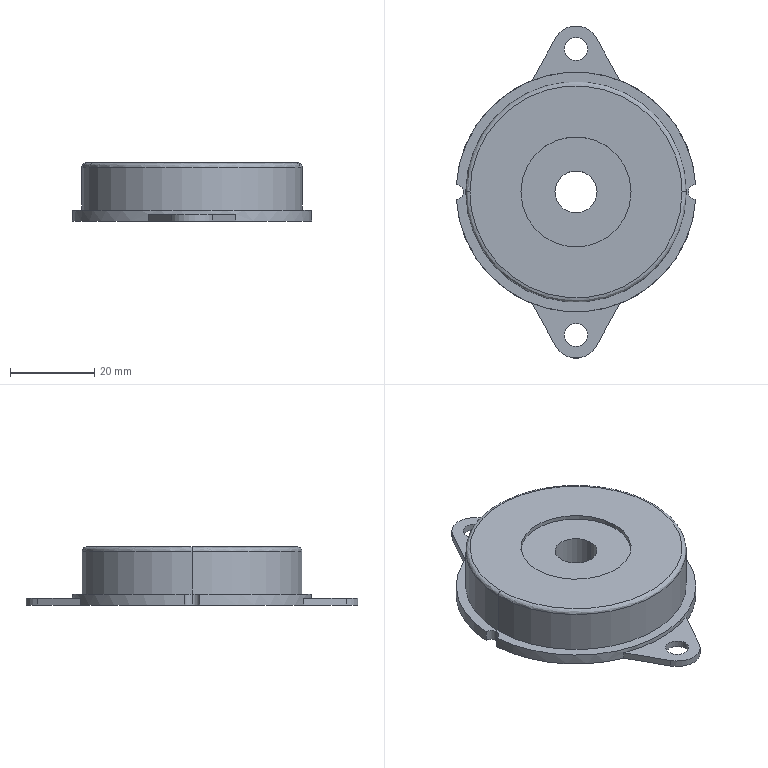Part | SolidWorks | features BaseBody 1 | 1 solid | 32 faces | box 56.886 x 79 x 13.8 mm | volume 28746 mm3 | cylinder 19 | plane 11 | spline 2 | commonest cylinder face diameters 5.5 x4 26.2 x4 3.6 x3 10 x2 11 x2 52.4 x2
STEP:
#1=CARTESIAN_POINT('',(26.2,0.,12.8));
#2=VERTEX_POINT('',#1);
#3=CARTESIAN_POINT('',(-26.2,0.,12.8));
#4=VERTEX_POINT('',#3);
#5=CARTESIAN_POINT('',(0.,0.,12.8));
#6=DIRECTION('',(0.,0.,-1.));
#7=DIRECTION('',(-1.,0.,0.));
#8=AXIS2_PLACEMENT_3D('',#5,#6,#7);
#9=CIRCLE('',#8,26.2);
#10=EDGE_CURVE('',#2,#4,#9,.T.);
#11=ORIENTED_EDGE('',*,*,#10,.F.);
#12=CARTESIAN_POINT('',(25.2,0.,13.8));
#13=VERTEX_POINT('',#12);
#14=CARTESIAN_POINT('',(25.2,0.,12.8));
#15=DIRECTION('',(0.,-1.,0.));
#16=DIRECTION('',(1.,0.,0.));
#17=AXIS2_PLACEMENT_3D('',#14,#15,#16);
#18=CIRCLE('',#17,1.);
#19=EDGE_CURVE('',#2,#13,#18,.T.);
#20=ORIENTED_EDGE('',*,*,#19,.T.);
#21=CARTESIAN_POINT('',(-25.2,0.,13.8));
#22=VERTEX_POINT('',#21);
#23=CARTESIAN_POINT('',(25.2,0.,13.8));
#24=CARTESIAN_POINT('',(25.2,-50.4,13.8));
#25=CARTESIAN_POINT('',(-25.2,-50.4,13.8));
#26=CARTESIAN_POINT('',(-25.2,0.,13.8));
#27=(BOUNDED_CURVE()B_SPLINE_CURVE(3,(#23,#24,#25,#26),.UNSPECIFIED.,.F.,.F.)B_SPLINE_CURVE_WITH_KNOTS((4,4),(0.5,1.),.UNSPECIFIED.)CURVE()GEOMETRIC_REPRESENTATION_ITEM()RATIONAL_B_SPLINE_CURVE((1.,0.3333,0.3333,1.))REPRESENTATION_ITEM(''));
#28=EDGE_CURVE('',#13,#22,#27,.T.);
#29=ORIENTED_EDGE('',*,*,#28,.T.);
#30=CARTESIAN_POINT('',(-25.2,0.,12.8));
#31=DIRECTION('',(0.,1.,0.));
#32=DIRECTION('',(-1.,0.,0.));
#33=AXIS2_PLACEMENT_3D('',#30,#31,#32);
#34=CIRCLE('',#33,1.);
#35=EDGE_CURVE('',#4,#22,#34,.T.);
#36=ORIENTED_EDGE('',*,*,#35,.F.);
#37=EDGE_LOOP('',(#11,#20,#29,#36));
#38=FACE_OUTER_BOUND('',#37,.T.);
#39=CARTESIAN_POINT('',(26.2,0.,12.8));
#40=CARTESIAN_POINT('',(26.2,-52.4,12.8));
#41=CARTESIAN_POINT('',(-26.2,-52.4,12.8));
#42=CARTESIAN_POINT('',(-26.2,0.,12.8));
#43=CARTESIAN_POINT('',(26.2,0.,13.386));
#44=CARTESIAN_POINT('',(26.2,-52.4,13.386));
#45=CARTESIAN_POINT('',(-26.2,-52.4,13.386));
#46=CARTESIAN_POINT('',(-26.2,0.,13.386));
#47=CARTESIAN_POINT('',(25.786,0.,13.8));
#48=CARTESIAN_POINT('',(25.786,-51.572,13.8));
#49=CARTESIAN_POINT('',(-25.786,-51.572,13.8));
#50=CARTESIAN_POINT('',(-25.786,0.,13.8));
#51=CARTESIAN_POINT('',(25.2,0.,13.8));
#52=CARTESIAN_POINT('',(25.2,-50.4,13.8));
#53=CARTESIAN_POINT('',(-25.2,-50.4,13.8));
#54=CARTESIAN_POINT('',(-25.2,0.,13.8));
#55=(BOUNDED_SURFACE()B_SPLINE_SURFACE(3,3,((#39,#40,#41,#42),(#43,#44,#45,#46),(#47,#48,#49,#50),(#51,#52,#53,#54)),.UNSPECIFIED.,.F.,.F.,.T.)B_SPLINE_SURFACE_WITH_KNOTS((4,4),(4,4),(0.,1.),(0.,1.),.UNSPECIFIED.)GEOMETRIC_REPRESENTATION_ITEM()RATIONAL_B_SPLINE_SURFACE(((1.,0.3333,0.3333,1.),(0.8047,0.2682,0.2682,0.8047),(0.8047,0.2682,0.2682,0.8047),(1.,0.3333,0.3333,1.)))REPRESENTATION_ITEM('')SURFACE());
#56=ADVANCED_FACE('',(#38),#55,.T.);
#57=CARTESIAN_POINT('',(-26.7,0.,0.));
#58=VERTEX_POINT('',#57);
#59=CARTESIAN_POINT('',(-28.443,1.799,0.));
#60=VERTEX_POINT('',#59);
#61=CARTESIAN_POINT('',(-28.5,0.,0.));
#62=DIRECTION('',(0.,0.,1.));
#63=DIRECTION('',(1.,0.,0.));
#64=AXIS2_PLACEMENT_3D('',#61,#62,#63);
#65=CIRCLE('',#64,1.8);
#66=EDGE_CURVE('',#58,#60,#65,.T.);
#67=ORIENTED_EDGE('',*,*,#66,.F.);
#68=CARTESIAN_POINT('',(-26.7,0.,2.6));
#69=VERTEX_POINT('',#68);
#70=CARTESIAN_POINT('',(-26.7,0.,-86.643));
#71=DIRECTION('',(0.,0.,1.));
#72=VECTOR('',#71,1000.);
#73=LINE('',#70,#72);
#74=EDGE_CURVE('',#58,#69,#73,.T.);
#75=ORIENTED_EDGE('',*,*,#74,.T.);
#76=CARTESIAN_POINT('',(-28.443,1.799,2.6));
#77=VERTEX_POINT('',#76);
#78=CARTESIAN_POINT('',(-28.5,0.,2.6));
#79=DIRECTION('',(0.,0.,-1.));
#80=DIRECTION('',(1.,0.,0.));
#81=AXIS2_PLACEMENT_3D('',#78,#79,#80);
#82=CIRCLE('',#81,1.8);
#83=EDGE_CURVE('',#77,#69,#82,.T.);
#84=ORIENTED_EDGE('',*,*,#83,.F.);
#85=CARTESIAN_POINT('',(-28.443,1.799,1.6));
#86=DIRECTION('',(0.,0.,1.));
#87=VECTOR('',#86,1000.);
#88=LINE('',#85,#87);
#89=EDGE_CURVE('',#60,#77,#88,.T.);
#90=ORIENTED_EDGE('',*,*,#89,.F.);
#91=EDGE_LOOP('',(#67,#75,#84,#90));
#92=FACE_OUTER_BOUND('',#91,.T.);
#93=CARTESIAN_POINT('',(-28.5,0.,-86.643));
#94=DIRECTION('',(0.,0.,1.));
#95=DIRECTION('',(1.,0.,0.));
#96=AXIS2_PLACEMENT_3D('',#93,#94,#95);
#97=CYLINDRICAL_SURFACE('',#96,1.8);
#98=ADVANCED_FACE('',(#92),#97,.F.);
#99=CARTESIAN_POINT('',(-2.75,34.,0.));
#100=VERTEX_POINT('',#99);
#101=CARTESIAN_POINT('',(2.75,34.,0.));
#102=VERTEX_POINT('',#101);
#103=CARTESIAN_POINT('',(0.,34.,0.));
#104=DIRECTION('',(0.,0.,1.));
#105=DIRECTION('',(1.,0.,0.));
#106=AXIS2_PLACEMENT_3D('',#103,#104,#105);
#107=CIRCLE('',#106,2.75);
#108=EDGE_CURVE('',#100,#102,#107,.T.);
#109=ORIENTED_EDGE('',*,*,#108,.F.);
#110=CARTESIAN_POINT('',(-2.75,34.,1.6));
#111=VERTEX_POINT('',#110);
#112=CARTESIAN_POINT('',(-2.75,34.,-84.589));
#113=DIRECTION('',(0.,0.,1.));
#114=VECTOR('',#113,1000.);
#115=LINE('',#112,#114);
#116=EDGE_CURVE('',#100,#111,#115,.T.);
#117=ORIENTED_EDGE('',*,*,#116,.T.);
#118=CARTESIAN_POINT('',(2.75,34.,1.6));
#119=VERTEX_POINT('',#118);
#120=CARTESIAN_POINT('',(0.,34.,1.6));
#121=DIRECTION('',(0.,0.,-1.));
#122=DIRECTION('',(1.,0.,0.));
#123=AXIS2_PLACEMENT_3D('',#120,#121,#122);
#124=CIRCLE('',#123,2.75);
#125=EDGE_CURVE('',#119,#111,#124,.T.);
#126=ORIENTED_EDGE('',*,*,#125,.F.);
#127=CARTESIAN_POINT('',(2.75,34.,-84.589));
#128=DIRECTION('',(0.,0.,1.));
#129=VECTOR('',#128,1000.);
#130=LINE('',#127,#129);
#131=EDGE_CURVE('',#102,#119,#130,.T.);
#132=ORIENTED_EDGE('',*,*,#131,.F.);
#133=EDGE_LOOP('',(#109,#117,#126,#132));
#134=FACE_OUTER_BOUND('',#133,.T.);
#135=CARTESIAN_POINT('',(0.,34.,-84.589));
#136=DIRECTION('',(0.,0.,1.));
#137=DIRECTION('',(1.,0.,0.));
#138=AXIS2_PLACEMENT_3D('',#135,#136,#137);
#139=CYLINDRICAL_SURFACE('',#138,2.75);
#140=ADVANCED_FACE('',(#134),#139,.F.);
#141=CARTESIAN_POINT('',(-2.75,-34.,0.));
#142=VERTEX_POINT('',#141);
#143=CARTESIAN_POINT('',(2.75,-34.,0.));
#144=VERTEX_POINT('',#143);
#145=CARTESIAN_POINT('',(0.,-34.,0.));
#146=DIRECTION('',(0.,0.,1.));
#147=DIRECTION('',(1.,0.,0.));
#148=AXIS2_PLACEMENT_3D('',#145,#146,#147);
#149=CIRCLE('',#148,2.75);
#150=EDGE_CURVE('',#142,#144,#149,.T.);
#151=ORIENTED_EDGE('',*,*,#150,.F.);
#152=CARTESIAN_POINT('',(-2.75,-34.,1.6));
#153=VERTEX_POINT('',#152);
#154=CARTESIAN_POINT('',(-2.75,-34.,-84.589));
#155=DIRECTION('',(0.,0.,1.));
#156=VECTOR('',#155,1000.);
#157=LINE('',#154,#156);
#158=EDGE_CURVE('',#142,#153,#157,.T.);
#159=ORIENTED_EDGE('',*,*,#158,.T.);
#160=CARTESIAN_POINT('',(2.75,-34.,1.6));
#161=VERTEX_POINT('',#160);
#162=CARTESIAN_POINT('',(0.,-34.,1.6));
#163=DIRECTION('',(0.,0.,-1.));
#164=DIRECTION('',(1.,0.,0.));
#165=AXIS2_PLACEMENT_3D('',#162,#163,#164);
#166=CIRCLE('',#165,2.75);
#167=EDGE_CURVE('',#161,#153,#166,.T.);
#168=ORIENTED_EDGE('',*,*,#167,.F.);
#169=CARTESIAN_POINT('',(2.75,-34.,-84.589));
#170=DIRECTION('',(0.,0.,1.));
#171=VECTOR('',#170,1000.);
#172=LINE('',#169,#171);
#173=EDGE_CURVE('',#144,#161,#172,.T.);
#174=ORIENTED_EDGE('',*,*,#173,.F.);
#175=EDGE_LOOP('',(#151,#159,#168,#174));
#176=FACE_OUTER_BOUND('',#175,.T.);
#177=CARTESIAN_POINT('',(0.,-34.,-84.589));
#178=DIRECTION('',(0.,0.,1.));
#179=DIRECTION('',(1.,0.,0.));
#180=AXIS2_PLACEMENT_3D('',#177,#178,#179);
#181=CYLINDRICAL_SURFACE('',#180,2.75);
#182=ADVANCED_FACE('',(#176),#181,.F.);
#183=CARTESIAN_POINT('',(13.1,0.,1.8));
#184=VERTEX_POINT('',#183);
#185=CARTESIAN_POINT('',(-13.1,0.,1.8));
#186=VERTEX_POINT('',#185);
#187=CARTESIAN_POINT('',(0.,0.,1.8));
#188=DIRECTION('',(0.,0.,-1.));
#189=DIRECTION('',(-1.,0.,0.));
#190=AXIS2_PLACEMENT_3D('',#187,#188,#189);
#191=CIRCLE('',#190,13.1);
#192=EDGE_CURVE('',#184,#186,#191,.T.);
#193=ORIENTED_EDGE('',*,*,#192,.F.);
#194=CARTESIAN_POINT('',(13.1,0.,0.));
#195=VERTEX_POINT('',#194);
#196=CARTESIAN_POINT('',(13.1,0.,1.8));
#197=DIRECTION('',(0.,0.,-1.));
#198=VECTOR('',#197,1000.);
#199=LINE('',#196,#198);
#200=EDGE_CURVE('',#184,#195,#199,.T.);
#201=ORIENTED_EDGE('',*,*,#200,.T.);
#202=CARTESIAN_POINT('',(-13.1,0.,0.));
#203=VERTEX_POINT('',#202);
#204=CARTESIAN_POINT('',(0.,0.,0.));
#205=DIRECTION('',(0.,0.,1.));
#206=DIRECTION('',(-1.,0.,0.));
#207=AXIS2_PLACEMENT_3D('',#204,#205,#206);
#208=CIRCLE('',#207,13.1);
#209=EDGE_CURVE('',#203,#195,#208,.T.);
#210=ORIENTED_EDGE('',*,*,#209,.F.);
#211=CARTESIAN_POINT('',(-13.1,0.,1.8));
#212=DIRECTION('',(0.,0.,-1.));
#213=VECTOR('',#212,1000.);
#214=LINE('',#211,#213);
#215=EDGE_CURVE('',#186,#203,#214,.T.);
#216=ORIENTED_EDGE('',*,*,#215,.F.);
#217=EDGE_LOOP('',(#193,#201,#210,#216));
#218=FACE_OUTER_BOUND('',#217,.T.);
#219=CARTESIAN_POINT('',(0.,0.,1.8));
#220=DIRECTION('',(0.,0.,-1.));
#221=DIRECTION('',(-1.,0.,0.));
#222=AXIS2_PLACEMENT_3D('',#219,#220,#221);
#223=CYLINDRICAL_SURFACE('',#222,13.1);
#224=ADVANCED_FACE('',(#218),#223,.F.);
#225=CARTESIAN_POINT('',(0.,0.,12.8));
#226=DIRECTION('',(0.,0.,-1.));
#227=DIRECTION('',(-1.,0.,0.));
#228=AXIS2_PLACEMENT_3D('',#225,#226,#227);
#229=CIRCLE('',#228,26.2);
#230=EDGE_CURVE('',#4,#2,#229,.T.);
#231=ORIENTED_EDGE('',*,*,#230,.T.);
#232=CARTESIAN_POINT('',(26.2,0.,2.6));
#233=VERTEX_POINT('',#232);
#234=CARTESIAN_POINT('',(26.2,0.,13.8));
#235=DIRECTION('',(0.,0.,-1.));
#236=VECTOR('',#235,1000.);
#237=LINE('',#234,#236);
#238=EDGE_CURVE('',#2,#233,#237,.T.);
#239=ORIENTED_EDGE('',*,*,#238,.T.);
#240=CARTESIAN_POINT('',(-26.2,0.,2.6));
#241=VERTEX_POINT('',#240);
#242=CARTESIAN_POINT('',(0.,0.,2.6));
#243=DIRECTION('',(0.,0.,1.));
#244=DIRECTION('',(-1.,0.,0.));
#245=AXIS2_PLACEMENT_3D('',#242,#243,#244);
#246=CIRCLE('',#245,26.2);
#247=EDGE_CURVE('',#233,#241,#246,.T.);
#248=ORIENTED_EDGE('',*,*,#247,.T.);
#249=CARTESIAN_POINT('',(-26.2,0.,13.8));
#250=DIRECTION('',(0.,0.,-1.));
#251=VECTOR('',#250,1000.);
#252=LINE('',#249,#251);
#253=EDGE_CURVE('',#4,#241,#252,.T.);
#254=ORIENTED_EDGE('',*,*,#253,.F.);
#255=EDGE_LOOP('',(#231,#239,#248,#254));
#256=FACE_OUTER_BOUND('',#255,.T.);
#257=CARTESIAN_POINT('',(0.,0.,13.8));
#258=DIRECTION('',(0.,0.,-1.));
#259=DIRECTION('',(-1.,0.,0.));
#260=AXIS2_PLACEMENT_3D('',#257,#258,#259);
#261=CYLINDRICAL_SURFACE('',#260,26.2);
#262=ADVANCED_FACE('',(#256),#261,.T.);
#263=CARTESIAN_POINT('',(5.,0.,1.8));
#264=VERTEX_POINT('',#263);
#265=CARTESIAN_POINT('',(-5.,0.,1.8));
#266=VERTEX_POINT('',#265);
#267=CARTESIAN_POINT('',(0.,0.,1.8));
#268=DIRECTION('',(0.,0.,-1.));
#269=DIRECTION('',(1.,0.,0.));
#270=AXIS2_PLACEMENT_3D('',#267,#268,#269);
#271=CIRCLE('',#270,5.);
#272=EDGE_CURVE('',#264,#266,#271,.T.);
#273=ORIENTED_EDGE('',*,*,#272,.T.);
#274=CARTESIAN_POINT('',(-5.,0.,12.8));
#275=VERTEX_POINT('',#274);
#276=CARTESIAN_POINT('',(-5.,0.,-84.589));
#277=DIRECTION('',(0.,0.,1.));
#278=VECTOR('',#277,1000.);
#279=LINE('',#276,#278);
#280=EDGE_CURVE('',#266,#275,#279,.T.);
#281=ORIENTED_EDGE('',*,*,#280,.T.);
#282=CARTESIAN_POINT('',(5.,0.,12.8));
#283=VERTEX_POINT('',#282);
#284=CARTESIAN_POINT('',(0.,0.,12.8));
#285=DIRECTION('',(0.,0.,-1.));
#286=DIRECTION('',(1.,0.,0.));
#287=AXIS2_PLACEMENT_3D('',#284,#285,#286);
#288=CIRCLE('',#287,5.);
#289=EDGE_CURVE('',#283,#275,#288,.T.);
#290=ORIENTED_EDGE('',*,*,#289,.F.);
#291=CARTESIAN_POINT('',(5.,0.,-84.589));
#292=DIRECTION('',(0.,0.,1.));
#293=VECTOR('',#292,1000.);
#294=LINE('',#291,#293);
#295=EDGE_CURVE('',#264,#283,#294,.T.);
#296=ORIENTED_EDGE('',*,*,#295,.F.);
#297=EDGE_LOOP('',(#273,#281,#290,#296));
#298=FACE_OUTER_BOUND('',#297,.T.);
#299=CARTESIAN_POINT('',(0.,0.,-84.589));
#300=DIRECTION('',(0.,0.,1.));
#301=DIRECTION('',(1.,0.,0.));
#302=AXIS2_PLACEMENT_3D('',#299,#300,#301);
#303=CYLINDRICAL_SURFACE('',#302,5.);
#304=ADVANCED_FACE('',(#298),#303,.F.);
#305=CARTESIAN_POINT('',(13.1,0.,12.8));
#306=VERTEX_POINT('',#305);
#307=CARTESIAN_POINT('',(-13.1,0.,12.8));
#308=VERTEX_POINT('',#307);
#309=CARTESIAN_POINT('',(0.,0.,12.8));
#310=DIRECTION('',(0.,0.,-1.));
#311=DIRECTION('',(1.,0.,0.));
#312=AXIS2_PLACEMENT_3D('',#309,#310,#311);
#313=CIRCLE('',#312,13.1);
#314=EDGE_CURVE('',#306,#308,#313,.T.);
#315=ORIENTED_EDGE('',*,*,#314,.T.);
#316=CARTESIAN_POINT('',(-13.1,0.,13.8));
#317=VERTEX_POINT('',#316);
#318=CARTESIAN_POINT('',(-13.1,0.,12.8));
#319=DIRECTION('',(0.,0.,1.));
#320=VECTOR('',#319,1000.);
#321=LINE('',#318,#320);
#322=EDGE_CURVE('',#308,#317,#321,.T.);
#323=ORIENTED_EDGE('',*,*,#322,.T.);
#324=CARTESIAN_POINT('',(13.1,0.,13.8));
#325=VERTEX_POINT('',#324);
#326=CARTESIAN_POINT('',(0.,0.,13.8));
#327=DIRECTION('',(0.,0.,1.));
#328=DIRECTION('',(1.,0.,0.));
#329=AXIS2_PLACEMENT_3D('',#326,#327,#328);
#330=CIRCLE('',#329,13.1);
#331=EDGE_CURVE('',#317,#325,#330,.T.);
#332=ORIENTED_EDGE('',*,*,#331,.T.);
#333=CARTESIAN_POINT('',(13.1,0.,12.8));
#334=DIRECTION('',(0.,0.,1.));
#335=VECTOR('',#334,1000.);
#336=LINE('',#333,#335);
#337=EDGE_CURVE('',#306,#325,#336,.T.);
#338=ORIENTED_EDGE('',*,*,#337,.F.);
#339=EDGE_LOOP('',(#315,#323,#332,#338));
#340=FACE_OUTER_BOUND('',#339,.T.);
#341=CARTESIAN_POINT('',(0.,0.,12.8));
#342=DIRECTION('',(0.,0.,1.));
#343=DIRECTION('',(1.,0.,0.));
#344=AXIS2_PLACEMENT_3D('',#341,#342,#343);
#345=CYLINDRICAL_SURFACE('',#344,13.1);
#346=ADVANCED_FACE('',(#340),#345,.F.);
#347=CARTESIAN_POINT('',(-4.81,36.666,0.));
#348=VERTEX_POINT('',#347);
#349=CARTESIAN_POINT('',(4.81,36.666,0.));
#350=VERTEX_POINT('',#349);
#351=CARTESIAN_POINT('',(0.,34.,0.));
#352=DIRECTION('',(0.,0.,-1.));
#353=DIRECTION('',(-1.,0.,0.));
#354=AXIS2_PLACEMENT_3D('',#351,#352,#353);
#355=CIRCLE('',#354,5.5);
#356=EDGE_CURVE('',#348,#350,#355,.T.);
#357=ORIENTED_EDGE('',*,*,#356,.T.);
#358=CARTESIAN_POINT('',(10.434,26.521,0.));
#359=VERTEX_POINT('',#358);
#360=CARTESIAN_POINT('',(4.81,36.666,0.));
#361=DIRECTION('',(0.4848,-0.8746,0.));
#362=VECTOR('',#361,1000.);
#363=LINE('',#360,#362);
#364=EDGE_CURVE('',#350,#359,#363,.T.);
#365=ORIENTED_EDGE('',*,*,#364,.T.);
#366=CARTESIAN_POINT('',(28.443,1.799,0.));
#367=VERTEX_POINT('',#366);
#368=CARTESIAN_POINT('',(0.,0.,0.));
#369=DIRECTION('',(0.,0.,-1.));
#370=DIRECTION('',(-1.,0.,0.));
#371=AXIS2_PLACEMENT_3D('',#368,#369,#370);
#372=CIRCLE('',#371,28.5);
#373=EDGE_CURVE('',#359,#367,#372,.T.);
#374=ORIENTED_EDGE('',*,*,#373,.T.);
#375=CARTESIAN_POINT('',(28.443,-1.799,0.));
#376=VERTEX_POINT('',#375);
#377=CARTESIAN_POINT('',(28.5,0.,0.));
#378=DIRECTION('',(0.,0.,1.));
#379=DIRECTION('',(1.,0.,0.));
#380=AXIS2_PLACEMENT_3D('',#377,#378,#379);
#381=CIRCLE('',#380,1.8);
#382=EDGE_CURVE('',#367,#376,#381,.T.);
#383=ORIENTED_EDGE('',*,*,#382,.T.);
#384=CARTESIAN_POINT('',(10.434,-26.521,0.));
#385=VERTEX_POINT('',#384);
#386=CARTESIAN_POINT('',(0.,0.,0.));
#387=DIRECTION('',(0.,0.,-1.));
#388=DIRECTION('',(-1.,0.,0.));
#389=AXIS2_PLACEMENT_3D('',#386,#387,#388);
#390=CIRCLE('',#389,28.5);
#391=EDGE_CURVE('',#376,#385,#390,.T.);
#392=ORIENTED_EDGE('',*,*,#391,.T.);
#393=CARTESIAN_POINT('',(4.81,-36.666,0.));
#394=VERTEX_POINT('',#393);
#395=CARTESIAN_POINT('',(10.434,-26.521,0.));
#396=DIRECTION('',(-0.4848,-0.8746,0.));
#397=VECTOR('',#396,1000.);
#398=LINE('',#395,#397);
#399=EDGE_CURVE('',#385,#394,#398,.T.);
#400=ORIENTED_EDGE('',*,*,#399,.T.);
#401=CARTESIAN_POINT('',(-4.81,-36.666,0.));
#402=VERTEX_POINT('',#401);
#403=CARTESIAN_POINT('',(0.,-34.,0.));
#404=DIRECTION('',(0.,0.,-1.));
#405=DIRECTION('',(-1.,0.,0.));
#406=AXIS2_PLACEMENT_3D('',#403,#404,#405);
#407=CIRCLE('',#406,5.5);
#408=EDGE_CURVE('',#394,#402,#407,.T.);
#409=ORIENTED_EDGE('',*,*,#408,.T.);
#410=CARTESIAN_POINT('',(-10.434,-26.521,0.));
#411=VERTEX_POINT('',#410);
#412=CARTESIAN_POINT('',(-4.81,-36.666,0.));
#413=DIRECTION('',(-0.4848,0.8746,0.));
#414=VECTOR('',#413,1000.);
#415=LINE('',#412,#414);
#416=EDGE_CURVE('',#402,#411,#415,.T.);
#417=ORIENTED_EDGE('',*,*,#416,.T.);
#418=CARTESIAN_POINT('',(-28.443,-1.799,0.));
#419=VERTEX_POINT('',#418);
#420=CARTESIAN_POINT('',(0.,0.,0.));
#421=DIRECTION('',(0.,0.,-1.));
#422=DIRECTION('',(-1.,0.,0.));
#423=AXIS2_PLACEMENT_3D('',#420,#421,#422);
#424=CIRCLE('',#423,28.5);
#425=EDGE_CURVE('',#411,#419,#424,.T.);
#426=ORIENTED_EDGE('',*,*,#425,.T.);
#427=CARTESIAN_POINT('',(-28.5,0.,0.));
#428=DIRECTION('',(0.,0.,1.));
#429=DIRECTION('',(1.,0.,0.));
#430=AXIS2_PLACEMENT_3D('',#427,#428,#429);
#431=CIRCLE('',#430,1.8);
#432=EDGE_CURVE('',#419,#58,#431,.T.);
#433=ORIENTED_EDGE('',*,*,#432,.T.);
#434=ORIENTED_EDGE('',*,*,#66,.T.);
#435=CARTESIAN_POINT('',(-10.434,26.521,0.));
#436=VERTEX_POINT('',#435);
#437=CARTESIAN_POINT('',(0.,0.,0.));
#438=DIRECTION('',(0.,0.,-1.));
#439=DIRECTION('',(-1.,0.,0.));
#440=AXIS2_PLACEMENT_3D('',#437,#438,#439);
#441=CIRCLE('',#440,28.5);
#442=EDGE_CURVE('',#60,#436,#441,.T.);
#443=ORIENTED_EDGE('',*,*,#442,.T.);
#444=CARTESIAN_POINT('',(-10.434,26.521,0.));
#445=DIRECTION('',(0.4848,0.8746,0.));
#446=VECTOR('',#445,1000.);
#447=LINE('',#444,#446);
#448=EDGE_CURVE('',#436,#348,#447,.T.);
#449=ORIENTED_EDGE('',*,*,#448,.T.);
#450=EDGE_LOOP('',(#357,#365,#374,#383,#392,#400,#409,#417,#426,#433,#434,#443,#449));
#451=FACE_OUTER_BOUND('',#450,.T.);
#452=CARTESIAN_POINT('',(0.,34.,0.));
#453=DIRECTION('',(0.,0.,1.));
#454=DIRECTION('',(1.,0.,0.));
#455=AXIS2_PLACEMENT_3D('',#452,#453,#454);
#456=CIRCLE('',#455,2.75);
#457=EDGE_CURVE('',#102,#100,#456,.T.);
#458=ORIENTED_EDGE('',*,*,#457,.T.);
#459=ORIENTED_EDGE('',*,*,#108,.T.);
#460=EDGE_LOOP('',(#458,#459));
#461=FACE_BOUND('',#460,.T.);
#462=CARTESIAN_POINT('',(0.,-34.,0.));
#463=DIRECTION('',(0.,0.,1.));
#464=DIRECTION('',(1.,0.,0.));
#465=AXIS2_PLACEMENT_3D('',#462,#463,#464);
#466=CIRCLE('',#465,2.75);
#467=EDGE_CURVE('',#144,#142,#466,.T.);
#468=ORIENTED_EDGE('',*,*,#467,.T.);
#469=ORIENTED_EDGE('',*,*,#150,.T.);
#470=EDGE_LOOP('',(#468,#469));
#471=FACE_BOUND('',#470,.T.);
#472=ORIENTED_EDGE('',*,*,#209,.T.);
#473=CARTESIAN_POINT('',(0.,0.,0.));
#474=DIRECTION('',(0.,0.,1.));
#475=DIRECTION('',(-1.,0.,0.));
#476=AXIS2_PLACEMENT_3D('',#473,#474,#475);
#477=CIRCLE('',#476,13.1);
#478=EDGE_CURVE('',#195,#203,#477,.T.);
#479=ORIENTED_EDGE('',*,*,#478,.T.);
#480=EDGE_LOOP('',(#472,#479));
#481=FACE_BOUND('',#480,.T.);
#482=CARTESIAN_POINT('',(0.,0.,0.));
#483=DIRECTION('',(0.,0.,-1.));
#484=DIRECTION('',(-1.,0.,0.));
#485=AXIS2_PLACEMENT_3D('',#482,#483,#484);
#486=PLANE('',#485);
#487=ADVANCED_FACE('',(#451,#461,#471,#481),#486,.T.);
#488=CARTESIAN_POINT('',(4.81,36.666,1.6));
#489=VERTEX_POINT('',#488);
#490=CARTESIAN_POINT('',(10.434,26.521,1.6));
#491=VERTEX_POINT('',#490);
#492=CARTESIAN_POINT('',(4.81,36.666,1.6));
#493=DIRECTION('',(0.4848,-0.8746,0.));
#494=VECTOR('',#493,1000.);
#495=LINE('',#492,#494);
#496=EDGE_CURVE('',#489,#491,#495,.T.);
#497=ORIENTED_EDGE('',*,*,#496,.T.);
#498=CARTESIAN_POINT('',(10.434,26.521,1.6));
#499=DIRECTION('',(0.,0.,-1.));
#500=VECTOR('',#499,1000.);
#501=LINE('',#498,#500);
#502=EDGE_CURVE('',#491,#359,#501,.T.);
#503=ORIENTED_EDGE('',*,*,#502,.T.);
#504=ORIENTED_EDGE('',*,*,#364,.F.);
#505=CARTESIAN_POINT('',(4.81,36.666,1.6));
#506=DIRECTION('',(0.,0.,1.));
#507=VECTOR('',#506,1000.);
#508=LINE('',#505,#507);
#509=EDGE_CURVE('',#350,#489,#508,.T.);
#510=ORIENTED_EDGE('',*,*,#509,.T.);
#511=EDGE_LOOP('',(#497,#503,#504,#510));
#512=FACE_OUTER_BOUND('',#511,.T.);
#513=CARTESIAN_POINT('',(4.81,36.666,1.6));
#514=DIRECTION('',(0.8746,0.4848,0.));
#515=DIRECTION('',(-0.4848,0.8746,0.));
#516=AXIS2_PLACEMENT_3D('',#513,#514,#515);
#517=PLANE('',#516);
#518=ADVANCED_FACE('',(#512),#517,.T.);
#519=CARTESIAN_POINT('',(-4.81,36.666,1.6));
#520=VERTEX_POINT('',#519);
#521=CARTESIAN_POINT('',(0.,34.,1.6));
#522=DIRECTION('',(0.,0.,-1.));
#523=DIRECTION('',(-1.,0.,0.));
#524=AXIS2_PLACEMENT_3D('',#521,#522,#523);
#525=CIRCLE('',#524,5.5);
#526=EDGE_CURVE('',#520,#489,#525,.T.);
#527=ORIENTED_EDGE('',*,*,#526,.T.);
#528=ORIENTED_EDGE('',*,*,#509,.F.);
#529=ORIENTED_EDGE('',*,*,#356,.F.);
#530=CARTESIAN_POINT('',(-4.81,36.666,1.6));
#531=DIRECTION('',(0.,0.,1.));
#532=VECTOR('',#531,1000.);
#533=LINE('',#530,#532);
#534=EDGE_CURVE('',#348,#520,#533,.T.);
#535=ORIENTED_EDGE('',*,*,#534,.T.);
#536=EDGE_LOOP('',(#527,#528,#529,#535));
#537=FACE_OUTER_BOUND('',#536,.T.);
#538=CARTESIAN_POINT('',(0.,34.,1.6));
#539=DIRECTION('',(0.,0.,-1.));
#540=DIRECTION('',(-1.,0.,0.));
#541=AXIS2_PLACEMENT_3D('',#538,#539,#540);
#542=CYLINDRICAL_SURFACE('',#541,5.5);
#543=ADVANCED_FACE('',(#537),#542,.T.);
#544=CARTESIAN_POINT('',(-10.434,26.521,1.6));
#545=VERTEX_POINT('',#544);
#546=CARTESIAN_POINT('',(-10.434,26.521,1.6));
#547=DIRECTION('',(0.4848,0.8746,0.));
#548=VECTOR('',#547,1000.);
#549=LINE('',#546,#548);
#550=EDGE_CURVE('',#545,#520,#549,.T.);
#551=ORIENTED_EDGE('',*,*,#550,.T.);
#552=ORIENTED_EDGE('',*,*,#534,.F.);
#553=ORIENTED_EDGE('',*,*,#448,.F.);
#554=CARTESIAN_POINT('',(-10.434,26.521,1.6));
#555=DIRECTION('',(0.,0.,1.));
#556=VECTOR('',#555,1000.);
#557=LINE('',#554,#556);
#558=EDGE_CURVE('',#436,#545,#557,.T.);
#559=ORIENTED_EDGE('',*,*,#558,.T.);
#560=EDGE_LOOP('',(#551,#552,#553,#559));
#561=FACE_OUTER_BOUND('',#560,.T.);
#562=CARTESIAN_POINT('',(-10.434,26.521,1.6));
#563=DIRECTION('',(-0.8746,0.4848,0.));
#564=DIRECTION('',(-0.4848,-0.8746,0.));
#565=AXIS2_PLACEMENT_3D('',#562,#563,#564);
#566=PLANE('',#565);
#567=ADVANCED_FACE('',(#561),#566,.T.);
#568=ORIENTED_EDGE('',*,*,#442,.F.);
#569=ORIENTED_EDGE('',*,*,#89,.T.);
#570=CARTESIAN_POINT('',(28.443,1.799,2.6));
#571=VERTEX_POINT('',#570);
#572=CARTESIAN_POINT('',(0.,0.,2.6));
#573=DIRECTION('',(0.,0.,-1.));
#574=DIRECTION('',(-1.,0.,0.));
#575=AXIS2_PLACEMENT_3D('',#572,#573,#574);
#576=CIRCLE('',#575,28.5);
#577=EDGE_CURVE('',#77,#571,#576,.T.);
#578=ORIENTED_EDGE('',*,*,#577,.T.);
#579=CARTESIAN_POINT('',(28.443,1.799,1.6));
#580=DIRECTION('',(0.,0.,-1.));
#581=VECTOR('',#580,1000.);
#582=LINE('',#579,#581);
#583=EDGE_CURVE('',#571,#367,#582,.T.);
#584=ORIENTED_EDGE('',*,*,#583,.T.);
#585=ORIENTED_EDGE('',*,*,#373,.F.);
#586=ORIENTED_EDGE('',*,*,#502,.F.);
#587=CARTESIAN_POINT('',(0.,0.,1.6));
#588=DIRECTION('',(0.,0.,1.));
#589=DIRECTION('',(-1.,0.,0.));
#590=AXIS2_PLACEMENT_3D('',#587,#588,#589);
#591=CIRCLE('',#590,28.5);
#592=EDGE_CURVE('',#491,#545,#591,.T.);
#593=ORIENTED_EDGE('',*,*,#592,.T.);
#594=ORIENTED_EDGE('',*,*,#558,.F.);
#595=EDGE_LOOP('',(#568,#569,#578,#584,#585,#586,#593,#594));
#596=FACE_OUTER_BOUND('',#595,.T.);
#597=CARTESIAN_POINT('',(0.,0.,1.6));
#598=DIRECTION('',(0.,0.,-1.));
#599=DIRECTION('',(-1.,0.,0.));
#600=AXIS2_PLACEMENT_3D('',#597,#598,#599);
#601=CYLINDRICAL_SURFACE('',#600,28.5);
#602=ADVANCED_FACE('',(#596),#601,.T.);
#603=ORIENTED_EDGE('',*,*,#74,.F.);
#604=ORIENTED_EDGE('',*,*,#432,.F.);
#605=CARTESIAN_POINT('',(-28.443,-1.799,2.6));
#606=VERTEX_POINT('',#605);
#607=CARTESIAN_POINT('',(-28.443,-1.799,-86.643));
#608=DIRECTION('',(0.,0.,-1.));
#609=VECTOR('',#608,1000.);
#610=LINE('',#607,#609);
#611=EDGE_CURVE('',#606,#419,#610,.T.);
#612=ORIENTED_EDGE('',*,*,#611,.F.);
#613=CARTESIAN_POINT('',(-28.5,0.,2.6));
#614=DIRECTION('',(0.,0.,-1.));
#615=DIRECTION('',(1.,0.,0.));
#616=AXIS2_PLACEMENT_3D('',#613,#614,#615);
#617=CIRCLE('',#616,1.8);
#618=EDGE_CURVE('',#69,#606,#617,.T.);
#619=ORIENTED_EDGE('',*,*,#618,.F.);
#620=EDGE_LOOP('',(#603,#604,#612,#619));
#621=FACE_OUTER_BOUND('',#620,.T.);
#622=CARTESIAN_POINT('',(-28.5,0.,-86.643));
#623=DIRECTION('',(0.,0.,1.));
#624=DIRECTION('',(1.,0.,0.));
#625=AXIS2_PLACEMENT_3D('',#622,#623,#624);
#626=CYLINDRICAL_SURFACE('',#625,1.8);
#627=ADVANCED_FACE('',(#621),#626,.F.);
#628=CARTESIAN_POINT('',(-10.434,-26.521,1.6));
#629=VERTEX_POINT('',#628);
#630=CARTESIAN_POINT('',(10.434,-26.521,1.6));
#631=VERTEX_POINT('',#630);
#632=CARTESIAN_POINT('',(0.,0.,1.6));
#633=DIRECTION('',(0.,0.,1.));
#634=DIRECTION('',(-1.,0.,0.));
#635=AXIS2_PLACEMENT_3D('',#632,#633,#634);
#636=CIRCLE('',#635,28.5);
#637=EDGE_CURVE('',#629,#631,#636,.T.);
#638=ORIENTED_EDGE('',*,*,#637,.T.);
#639=CARTESIAN_POINT('',(10.434,-26.521,1.6));
#640=DIRECTION('',(0.,0.,-1.));
#641=VECTOR('',#640,1000.);
#642=LINE('',#639,#641);
#643=EDGE_CURVE('',#631,#385,#642,.T.);
#644=ORIENTED_EDGE('',*,*,#643,.T.);
#645=ORIENTED_EDGE('',*,*,#391,.F.);
#646=CARTESIAN_POINT('',(28.443,-1.799,2.6));
#647=VERTEX_POINT('',#646);
#648=CARTESIAN_POINT('',(28.443,-1.799,1.6));
#649=DIRECTION('',(0.,0.,1.));
#650=VECTOR('',#649,1000.);
#651=LINE('',#648,#650);
#652=EDGE_CURVE('',#376,#647,#651,.T.);
#653=ORIENTED_EDGE('',*,*,#652,.T.);
#654=CARTESIAN_POINT('',(0.,0.,2.6));
#655=DIRECTION('',(0.,0.,-1.));
#656=DIRECTION('',(-1.,0.,0.));
#657=AXIS2_PLACEMENT_3D('',#654,#655,#656);
#658=CIRCLE('',#657,28.5);
#659=EDGE_CURVE('',#647,#606,#658,.T.);
#660=ORIENTED_EDGE('',*,*,#659,.T.);
#661=ORIENTED_EDGE('',*,*,#611,.T.);
#662=ORIENTED_EDGE('',*,*,#425,.F.);
#663=CARTESIAN_POINT('',(-10.434,-26.521,1.6));
#664=DIRECTION('',(0.,0.,1.));
#665=VECTOR('',#664,1000.);
#666=LINE('',#663,#665);
#667=EDGE_CURVE('',#411,#629,#666,.T.);
#668=ORIENTED_EDGE('',*,*,#667,.T.);
#669=EDGE_LOOP('',(#638,#644,#645,#653,#660,#661,#662,#668));
#670=FACE_OUTER_BOUND('',#669,.T.);
#671=CARTESIAN_POINT('',(0.,0.,1.6));
#672=DIRECTION('',(0.,0.,-1.));
#673=DIRECTION('',(-1.,0.,0.));
#674=AXIS2_PLACEMENT_3D('',#671,#672,#673);
#675=CYLINDRICAL_SURFACE('',#674,28.5);
#676=ADVANCED_FACE('',(#670),#675,.T.);
#677=CARTESIAN_POINT('',(-4.81,-36.666,1.6));
#678=VERTEX_POINT('',#677);
#679=CARTESIAN_POINT('',(-10.434,-26.521,1.6));
#680=DIRECTION('',(-0.4848,0.8746,0.));
#681=VECTOR('',#680,1000.);
#682=LINE('',#679,#681);
#683=EDGE_CURVE('',#678,#629,#682,.T.);
#684=ORIENTED_EDGE('',*,*,#683,.T.);
#685=ORIENTED_EDGE('',*,*,#667,.F.);
#686=ORIENTED_EDGE('',*,*,#416,.F.);
#687=CARTESIAN_POINT('',(-4.81,-36.666,1.6));
#688=DIRECTION('',(0.,0.,1.));
#689=VECTOR('',#688,1000.);
#690=LINE('',#687,#689);
#691=EDGE_CURVE('',#402,#678,#690,.T.);
#692=ORIENTED_EDGE('',*,*,#691,.T.);
#693=EDGE_LOOP('',(#684,#685,#686,#692));
#694=FACE_OUTER_BOUND('',#693,.T.);
#695=CARTESIAN_POINT('',(-10.434,-26.521,1.6));
#696=DIRECTION('',(-0.8746,-0.4848,0.));
#697=DIRECTION('',(0.4848,-0.8746,0.));
#698=AXIS2_PLACEMENT_3D('',#695,#696,#697);
#699=PLANE('',#698);
#700=ADVANCED_FACE('',(#694),#699,.T.);
#701=CARTESIAN_POINT('',(4.81,-36.666,1.6));
#702=VERTEX_POINT('',#701);
#703=CARTESIAN_POINT('',(0.,-34.,1.6));
#704=DIRECTION('',(0.,0.,-1.));
#705=DIRECTION('',(-1.,0.,0.));
#706=AXIS2_PLACEMENT_3D('',#703,#704,#705);
#707=CIRCLE('',#706,5.5);
#708=EDGE_CURVE('',#702,#678,#707,.T.);
#709=ORIENTED_EDGE('',*,*,#708,.T.);
#710=ORIENTED_EDGE('',*,*,#691,.F.);
#711=ORIENTED_EDGE('',*,*,#408,.F.);
#712=CARTESIAN_POINT('',(4.81,-36.666,1.6));
#713=DIRECTION('',(0.,0.,1.));
#714=VECTOR('',#713,1000.);
#715=LINE('',#712,#714);
#716=EDGE_CURVE('',#394,#702,#715,.T.);
#717=ORIENTED_EDGE('',*,*,#716,.T.);
#718=EDGE_LOOP('',(#709,#710,#711,#717));
#719=FACE_OUTER_BOUND('',#718,.T.);
#720=CARTESIAN_POINT('',(0.,-34.,1.6));
#721=DIRECTION('',(0.,0.,-1.));
#722=DIRECTION('',(-1.,0.,0.));
#723=AXIS2_PLACEMENT_3D('',#720,#721,#722);
#724=CYLINDRICAL_SURFACE('',#723,5.5);
#725=ADVANCED_FACE('',(#719),#724,.T.);
#726=CARTESIAN_POINT('',(4.81,-36.666,1.6));
#727=DIRECTION('',(-0.4848,-0.8746,0.));
#728=VECTOR('',#727,1000.);
#729=LINE('',#726,#728);
#730=EDGE_CURVE('',#631,#702,#729,.T.);
#731=ORIENTED_EDGE('',*,*,#730,.T.);
#732=ORIENTED_EDGE('',*,*,#716,.F.);
#733=ORIENTED_EDGE('',*,*,#399,.F.);
#734=ORIENTED_EDGE('',*,*,#643,.F.);
#735=EDGE_LOOP('',(#731,#732,#733,#734));
#736=FACE_OUTER_BOUND('',#735,.T.);
#737=CARTESIAN_POINT('',(4.81,-36.666,1.6));
#738=DIRECTION('',(0.8746,-0.4848,0.));
#739=DIRECTION('',(0.4848,0.8746,0.));
#740=AXIS2_PLACEMENT_3D('',#737,#738,#739);
#741=PLANE('',#740);
#742=ADVANCED_FACE('',(#736),#741,.T.);
#743=CARTESIAN_POINT('',(28.5,0.,2.6));
#744=DIRECTION('',(0.,0.,-1.));
#745=DIRECTION('',(1.,0.,0.));
#746=AXIS2_PLACEMENT_3D('',#743,#744,#745);
#747=CIRCLE('',#746,1.8);
#748=EDGE_CURVE('',#647,#571,#747,.T.);
#749=ORIENTED_EDGE('',*,*,#748,.F.);
#750=ORIENTED_EDGE('',*,*,#652,.F.);
#751=ORIENTED_EDGE('',*,*,#382,.F.);
#752=ORIENTED_EDGE('',*,*,#583,.F.);
#753=EDGE_LOOP('',(#749,#750,#751,#752));
#754=FACE_OUTER_BOUND('',#753,.T.);
#755=CARTESIAN_POINT('',(28.5,0.,-86.609));
#756=DIRECTION('',(0.,0.,1.));
#757=DIRECTION('',(1.,0.,0.));
#758=AXIS2_PLACEMENT_3D('',#755,#756,#757);
#759=CYLINDRICAL_SURFACE('',#758,1.8);
#760=ADVANCED_FACE('',(#754),#759,.F.);
#761=ORIENTED_EDGE('',*,*,#116,.F.);
#762=ORIENTED_EDGE('',*,*,#457,.F.);
#763=ORIENTED_EDGE('',*,*,#131,.T.);
#764=CARTESIAN_POINT('',(0.,34.,1.6));
#765=DIRECTION('',(0.,0.,-1.));
#766=DIRECTION('',(1.,0.,0.));
#767=AXIS2_PLACEMENT_3D('',#764,#765,#766);
#768=CIRCLE('',#767,2.75);
#769=EDGE_CURVE('',#111,#119,#768,.T.);
#770=ORIENTED_EDGE('',*,*,#769,.F.);
#771=EDGE_LOOP('',(#761,#762,#763,#770));
#772=FACE_OUTER_BOUND('',#771,.T.);
#773=CARTESIAN_POINT('',(0.,34.,-84.589));
#774=DIRECTION('',(0.,0.,1.));
#775=DIRECTION('',(1.,0.,0.));
#776=AXIS2_PLACEMENT_3D('',#773,#774,#775);
#777=CYLINDRICAL_SURFACE('',#776,2.75);
#778=ADVANCED_FACE('',(#772),#777,.F.);
#779=ORIENTED_EDGE('',*,*,#158,.F.);
#780=ORIENTED_EDGE('',*,*,#467,.F.);
#781=ORIENTED_EDGE('',*,*,#173,.T.);
#782=CARTESIAN_POINT('',(0.,-34.,1.6));
#783=DIRECTION('',(0.,0.,-1.));
#784=DIRECTION('',(1.,0.,0.));
#785=AXIS2_PLACEMENT_3D('',#782,#783,#784);
#786=CIRCLE('',#785,2.75);
#787=EDGE_CURVE('',#153,#161,#786,.T.);
#788=ORIENTED_EDGE('',*,*,#787,.F.);
#789=EDGE_LOOP('',(#779,#780,#781,#788));
#790=FACE_OUTER_BOUND('',#789,.T.);
#791=CARTESIAN_POINT('',(0.,-34.,-84.589));
#792=DIRECTION('',(0.,0.,1.));
#793=DIRECTION('',(1.,0.,0.));
#794=AXIS2_PLACEMENT_3D('',#791,#792,#793);
#795=CYLINDRICAL_SURFACE('',#794,2.75);
#796=ADVANCED_FACE('',(#790),#795,.F.);
#797=ORIENTED_EDGE('',*,*,#200,.F.);
#798=CARTESIAN_POINT('',(0.,0.,1.8));
#799=DIRECTION('',(0.,0.,-1.));
#800=DIRECTION('',(-1.,0.,0.));
#801=AXIS2_PLACEMENT_3D('',#798,#799,#800);
#802=CIRCLE('',#801,13.1);
#803=EDGE_CURVE('',#186,#184,#802,.T.);
#804=ORIENTED_EDGE('',*,*,#803,.F.);
#805=ORIENTED_EDGE('',*,*,#215,.T.);
#806=ORIENTED_EDGE('',*,*,#478,.F.);
#807=EDGE_LOOP('',(#797,#804,#805,#806));
#808=FACE_OUTER_BOUND('',#807,.T.);
#809=CARTESIAN_POINT('',(0.,0.,1.8));
#810=DIRECTION('',(0.,0.,-1.));
#811=DIRECTION('',(-1.,0.,0.));
#812=AXIS2_PLACEMENT_3D('',#809,#810,#811);
#813=CYLINDRICAL_SURFACE('',#812,13.1);
#814=ADVANCED_FACE('',(#808),#813,.F.);
#815=ORIENTED_EDGE('',*,*,#592,.F.);
#816=ORIENTED_EDGE('',*,*,#496,.F.);
#817=ORIENTED_EDGE('',*,*,#526,.F.);
#818=ORIENTED_EDGE('',*,*,#550,.F.);
#819=EDGE_LOOP('',(#815,#816,#817,#818));
#820=FACE_OUTER_BOUND('',#819,.T.);
#821=ORIENTED_EDGE('',*,*,#125,.T.);
#822=ORIENTED_EDGE('',*,*,#769,.T.);
#823=EDGE_LOOP('',(#821,#822));
#824=FACE_BOUND('',#823,.T.);
#825=CARTESIAN_POINT('',(0.,0.,1.6));
#826=DIRECTION('',(0.,0.,-1.));
#827=DIRECTION('',(-1.,0.,0.));
#828=AXIS2_PLACEMENT_3D('',#825,#826,#827);
#829=PLANE('',#828);
#830=ADVANCED_FACE('',(#820,#824),#829,.F.);
#831=CARTESIAN_POINT('',(0.,0.,2.6));
#832=DIRECTION('',(0.,0.,1.));
#833=DIRECTION('',(-1.,0.,0.));
#834=AXIS2_PLACEMENT_3D('',#831,#832,#833);
#835=CIRCLE('',#834,26.2);
#836=EDGE_CURVE('',#241,#233,#835,.T.);
#837=ORIENTED_EDGE('',*,*,#836,.F.);
#838=ORIENTED_EDGE('',*,*,#247,.F.);
#839=EDGE_LOOP('',(#837,#838));
#840=FACE_BOUND('',#839,.T.);
#841=ORIENTED_EDGE('',*,*,#577,.F.);
#842=ORIENTED_EDGE('',*,*,#83,.T.);
#843=ORIENTED_EDGE('',*,*,#618,.T.);
#844=ORIENTED_EDGE('',*,*,#659,.F.);
#845=ORIENTED_EDGE('',*,*,#748,.T.);
#846=EDGE_LOOP('',(#841,#842,#843,#844,#845));
#847=FACE_OUTER_BOUND('',#846,.T.);
#848=CARTESIAN_POINT('',(0.,0.,2.6));
#849=DIRECTION('',(0.,0.,-1.));
#850=DIRECTION('',(-1.,0.,0.));
#851=AXIS2_PLACEMENT_3D('',#848,#849,#850);
#852=PLANE('',#851);
#853=ADVANCED_FACE('',(#840,#847),#852,.F.);
#854=ORIENTED_EDGE('',*,*,#637,.F.);
#855=ORIENTED_EDGE('',*,*,#683,.F.);
#856=ORIENTED_EDGE('',*,*,#708,.F.);
#857=ORIENTED_EDGE('',*,*,#730,.F.);
#858=EDGE_LOOP('',(#854,#855,#856,#857));
#859=FACE_OUTER_BOUND('',#858,.T.);
#860=ORIENTED_EDGE('',*,*,#167,.T.);
#861=ORIENTED_EDGE('',*,*,#787,.T.);
#862=EDGE_LOOP('',(#860,#861));
#863=FACE_BOUND('',#862,.T.);
#864=CARTESIAN_POINT('',(0.,0.,1.6));
#865=DIRECTION('',(0.,0.,-1.));
#866=DIRECTION('',(-1.,0.,0.));
#867=AXIS2_PLACEMENT_3D('',#864,#865,#866);
#868=PLANE('',#867);
#869=ADVANCED_FACE('',(#859,#863),#868,.F.);
#870=ORIENTED_EDGE('',*,*,#803,.T.);
#871=ORIENTED_EDGE('',*,*,#192,.T.);
#872=EDGE_LOOP('',(#870,#871));
#873=FACE_OUTER_BOUND('',#872,.T.);
#874=ORIENTED_EDGE('',*,*,#272,.F.);
#875=CARTESIAN_POINT('',(0.,0.,1.8));
#876=DIRECTION('',(0.,0.,-1.));
#877=DIRECTION('',(1.,0.,0.));
#878=AXIS2_PLACEMENT_3D('',#875,#876,#877);
#879=CIRCLE('',#878,5.);
#880=EDGE_CURVE('',#266,#264,#879,.T.);
#881=ORIENTED_EDGE('',*,*,#880,.F.);
#882=EDGE_LOOP('',(#874,#881));
#883=FACE_BOUND('',#882,.T.);
#884=CARTESIAN_POINT('',(0.,0.,1.8));
#885=DIRECTION('',(0.,0.,1.));
#886=DIRECTION('',(1.,0.,0.));
#887=AXIS2_PLACEMENT_3D('',#884,#885,#886);
#888=PLANE('',#887);
#889=ADVANCED_FACE('',(#873,#883),#888,.F.);
#890=ORIENTED_EDGE('',*,*,#238,.F.);
#891=ORIENTED_EDGE('',*,*,#10,.T.);
#892=ORIENTED_EDGE('',*,*,#253,.T.);
#893=ORIENTED_EDGE('',*,*,#836,.T.);
#894=EDGE_LOOP('',(#890,#891,#892,#893));
#895=FACE_OUTER_BOUND('',#894,.T.);
#896=CARTESIAN_POINT('',(0.,0.,13.8));
#897=DIRECTION('',(0.,0.,-1.));
#898=DIRECTION('',(-1.,0.,0.));
#899=AXIS2_PLACEMENT_3D('',#896,#897,#898);
#900=CYLINDRICAL_SURFACE('',#899,26.2);
#901=ADVANCED_FACE('',(#895),#900,.T.);
#902=ORIENTED_EDGE('',*,*,#280,.F.);
#903=ORIENTED_EDGE('',*,*,#880,.T.);
#904=ORIENTED_EDGE('',*,*,#295,.T.);
#905=CARTESIAN_POINT('',(0.,0.,12.8));
#906=DIRECTION('',(0.,0.,-1.));
#907=DIRECTION('',(1.,0.,0.));
#908=AXIS2_PLACEMENT_3D('',#905,#906,#907);
#909=CIRCLE('',#908,5.);
#910=EDGE_CURVE('',#275,#283,#909,.T.);
#911=ORIENTED_EDGE('',*,*,#910,.F.);
#912=EDGE_LOOP('',(#902,#903,#904,#911));
#913=FACE_OUTER_BOUND('',#912,.T.);
#914=CARTESIAN_POINT('',(0.,0.,-84.589));
#915=DIRECTION('',(0.,0.,1.));
#916=DIRECTION('',(1.,0.,0.));
#917=AXIS2_PLACEMENT_3D('',#914,#915,#916);
#918=CYLINDRICAL_SURFACE('',#917,5.);
#919=ADVANCED_FACE('',(#913),#918,.F.);
#920=ORIENTED_EDGE('',*,*,#19,.F.);
#921=ORIENTED_EDGE('',*,*,#230,.F.);
#922=ORIENTED_EDGE('',*,*,#35,.T.);
#923=CARTESIAN_POINT('',(-25.2,0.,13.8));
#924=CARTESIAN_POINT('',(-25.2,50.4,13.8));
#925=CARTESIAN_POINT('',(25.2,50.4,13.8));
#926=CARTESIAN_POINT('',(25.2,0.,13.8));
#927=(BOUNDED_CURVE()B_SPLINE_CURVE(3,(#923,#924,#925,#926),.UNSPECIFIED.,.F.,.F.)B_SPLINE_CURVE_WITH_KNOTS((4,4),(0.,0.5),.UNSPECIFIED.)CURVE()GEOMETRIC_REPRESENTATION_ITEM()RATIONAL_B_SPLINE_CURVE((1.,0.3333,0.3333,1.))REPRESENTATION_ITEM(''));
#928=EDGE_CURVE('',#22,#13,#927,.T.);
#929=ORIENTED_EDGE('',*,*,#928,.T.);
#930=EDGE_LOOP('',(#920,#921,#922,#929));
#931=FACE_OUTER_BOUND('',#930,.T.);
#932=CARTESIAN_POINT('',(-26.2,0.,12.8));
#933=CARTESIAN_POINT('',(-26.2,52.4,12.8));
#934=CARTESIAN_POINT('',(26.2,52.4,12.8));
#935=CARTESIAN_POINT('',(26.2,0.,12.8));
#936=CARTESIAN_POINT('',(-26.2,0.,13.386));
#937=CARTESIAN_POINT('',(-26.2,52.4,13.386));
#938=CARTESIAN_POINT('',(26.2,52.4,13.386));
#939=CARTESIAN_POINT('',(26.2,0.,13.386));
#940=CARTESIAN_POINT('',(-25.786,0.,13.8));
#941=CARTESIAN_POINT('',(-25.786,51.572,13.8));
#942=CARTESIAN_POINT('',(25.786,51.572,13.8));
#943=CARTESIAN_POINT('',(25.786,0.,13.8));
#944=CARTESIAN_POINT('',(-25.2,0.,13.8));
#945=CARTESIAN_POINT('',(-25.2,50.4,13.8));
#946=CARTESIAN_POINT('',(25.2,50.4,13.8));
#947=CARTESIAN_POINT('',(25.2,0.,13.8));
#948=(BOUNDED_SURFACE()B_SPLINE_SURFACE(3,3,((#932,#933,#934,#935),(#936,#937,#938,#939),(#940,#941,#942,#943),(#944,#945,#946,#947)),.UNSPECIFIED.,.F.,.F.,.T.)B_SPLINE_SURFACE_WITH_KNOTS((4,4),(4,4),(0.,1.),(0.,1.),.UNSPECIFIED.)GEOMETRIC_REPRESENTATION_ITEM()RATIONAL_B_SPLINE_SURFACE(((1.,0.3333,0.3333,1.),(0.8047,0.2682,0.2682,0.8047),(0.8047,0.2682,0.2682,0.8047),(1.,0.3333,0.3333,1.)))REPRESENTATION_ITEM('')SURFACE());
#949=ADVANCED_FACE('',(#931),#948,.T.);
#950=ORIENTED_EDGE('',*,*,#314,.F.);
#951=CARTESIAN_POINT('',(0.,0.,12.8));
#952=DIRECTION('',(0.,0.,-1.));
#953=DIRECTION('',(1.,0.,0.));
#954=AXIS2_PLACEMENT_3D('',#951,#952,#953);
#955=CIRCLE('',#954,13.1);
#956=EDGE_CURVE('',#308,#306,#955,.T.);
#957=ORIENTED_EDGE('',*,*,#956,.F.);
#958=EDGE_LOOP('',(#950,#957));
#959=FACE_OUTER_BOUND('',#958,.T.);
#960=ORIENTED_EDGE('',*,*,#289,.T.);
#961=ORIENTED_EDGE('',*,*,#910,.T.);
#962=EDGE_LOOP('',(#960,#961));
#963=FACE_BOUND('',#962,.T.);
#964=CARTESIAN_POINT('',(0.,0.,12.8));
#965=DIRECTION('',(0.,0.,-1.));
#966=DIRECTION('',(-1.,0.,0.));
#967=AXIS2_PLACEMENT_3D('',#964,#965,#966);
#968=PLANE('',#967);
#969=ADVANCED_FACE('',(#959,#963),#968,.F.);
#970=ORIENTED_EDGE('',*,*,#928,.F.);
#971=ORIENTED_EDGE('',*,*,#28,.F.);
#972=EDGE_LOOP('',(#970,#971));
#973=FACE_OUTER_BOUND('',#972,.T.);
#974=CARTESIAN_POINT('',(0.,0.,13.8));
#975=DIRECTION('',(0.,0.,1.));
#976=DIRECTION('',(1.,0.,0.));
#977=AXIS2_PLACEMENT_3D('',#974,#975,#976);
#978=CIRCLE('',#977,13.1);
#979=EDGE_CURVE('',#325,#317,#978,.T.);
#980=ORIENTED_EDGE('',*,*,#979,.F.);
#981=ORIENTED_EDGE('',*,*,#331,.F.);
#982=EDGE_LOOP('',(#980,#981));
#983=FACE_BOUND('',#982,.T.);
#984=CARTESIAN_POINT('',(0.,0.,13.8));
#985=DIRECTION('',(0.,0.,-1.));
#986=DIRECTION('',(-1.,0.,0.));
#987=AXIS2_PLACEMENT_3D('',#984,#985,#986);
#988=PLANE('',#987);
#989=ADVANCED_FACE('',(#973,#983),#988,.F.);
#990=ORIENTED_EDGE('',*,*,#322,.F.);
#991=ORIENTED_EDGE('',*,*,#956,.T.);
#992=ORIENTED_EDGE('',*,*,#337,.T.);
#993=ORIENTED_EDGE('',*,*,#979,.T.);
#994=EDGE_LOOP('',(#990,#991,#992,#993));
#995=FACE_OUTER_BOUND('',#994,.T.);
#996=CARTESIAN_POINT('',(0.,0.,12.8));
#997=DIRECTION('',(0.,0.,1.));
#998=DIRECTION('',(1.,0.,0.));
#999=AXIS2_PLACEMENT_3D('',#996,#997,#998);
#1000=CYLINDRICAL_SURFACE('',#999,13.1);
#1001=ADVANCED_FACE('',(#995),#1000,.F.);
#1002=CLOSED_SHELL('',(#56,#98,#140,#182,#224,#262,#304,#346,#487,#518,#543,#567,#602,#627,#676,#700,#725,#742,#760,#778,#796,#814,#830,#853,#869,#889,#901,#919,#949,#969,#989,#1001));
#1003=MANIFOLD_SOLID_BREP('',#1002);
#1004=CARTESIAN_POINT('',(0.,0.,0.));
#1005=DIRECTION('',(0.,0.,1.));
#1006=DIRECTION('',(1.,0.,0.));
#1007=AXIS2_PLACEMENT_3D('',#1004,#1005,#1006);
#1008=(LENGTH_UNIT()NAMED_UNIT(*)SI_UNIT(.MILLI.,.METRE.));
#1009=UNCERTAINTY_MEASURE_WITH_UNIT(LENGTH_MEASURE(0.00001),#1008,'','');
#1010=(NAMED_UNIT(*)PLANE_ANGLE_UNIT()SI_UNIT($,.RADIAN.));
#1011=(NAMED_UNIT(*)SI_UNIT($,.STERADIAN.)SOLID_ANGLE_UNIT());
#1012=(GEOMETRIC_REPRESENTATION_CONTEXT(3)GLOBAL_UNCERTAINTY_ASSIGNED_CONTEXT((#1009))GLOBAL_UNIT_ASSIGNED_CONTEXT((#1008,#1010,#1011))REPRESENTATION_CONTEXT('',''));
#1013=ADVANCED_BREP_SHAPE_REPRESENTATION('',(#1003,#1007),#1012);